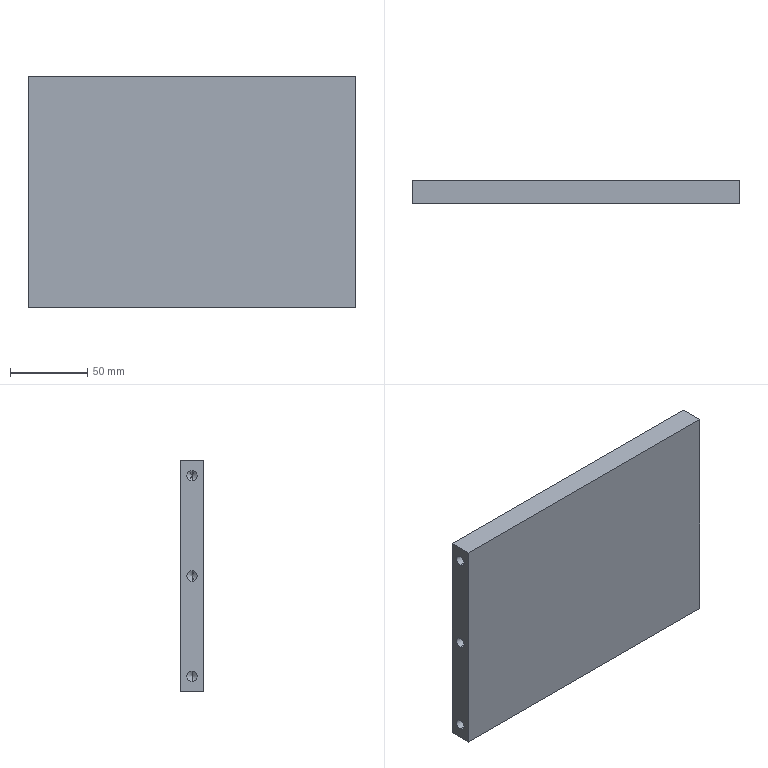Part | STEP file | CON-020 | 1 solid | 30 faces | box 212 x 15 x 150 mm | volume 472548 mm3 | cylinder 12 | cone 12 | plane 6 | commonest cylinder face diameters 6.8 x12